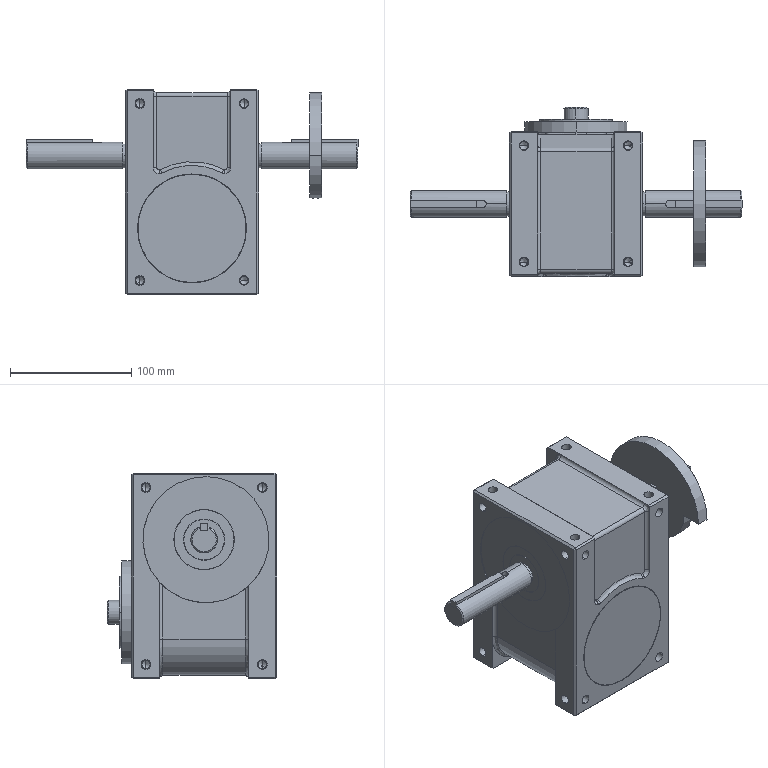Part | SolidWorks | 5 solids | 873 faces | box 274 x 140 x 170 mm | volume 2243698 mm3 | cylinder 408 | plane 331 | cone 103 | spline 31 | commonest cylinder face diameters 8 x240 6.8 x48 5 x26 1 x22 6 x20 104 x10